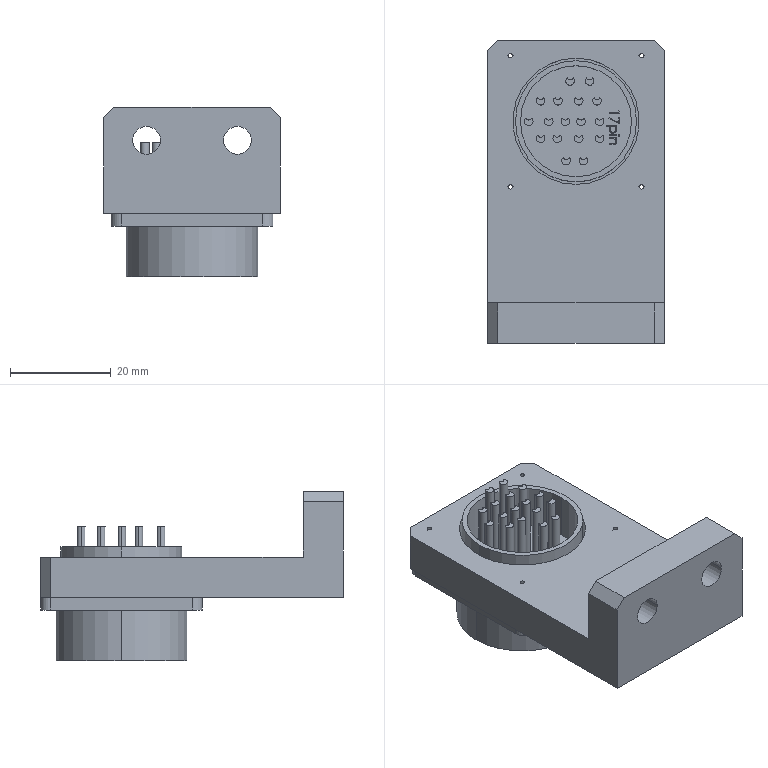Part | NX | features BREP 2 | 2 solids | 324 faces | box 35 x 60 x 33.5 mm | volume 21218 mm3 | plane 148 | cylinder 144 | spline 24 | cone 8 | commonest cylinder face diameters 1.7 x51 1 x35 1.243 x17 2.5 x8 3.5 x8 4 x4